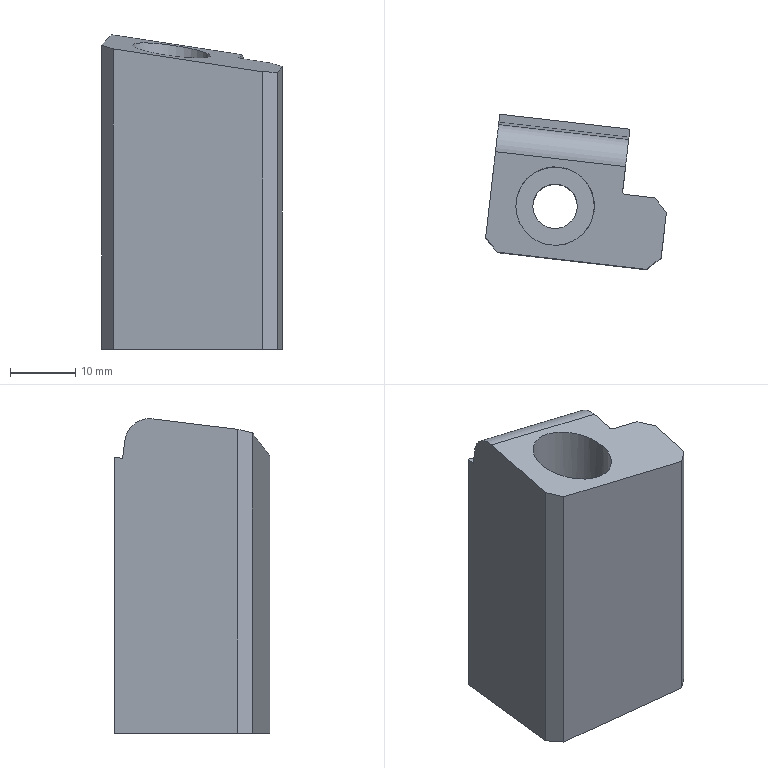Part | STEP file | gslz 2016.10.28-13_id1534_x_t | 1 solid | 18 faces | box 27.622 x 23.712 x 48.072 mm | volume 19234 mm3 | plane 11 | cylinder 4 | spline 3 | commonest cylinder face diameters 1 x1 6.8 x1 7.5 x1 12 x1